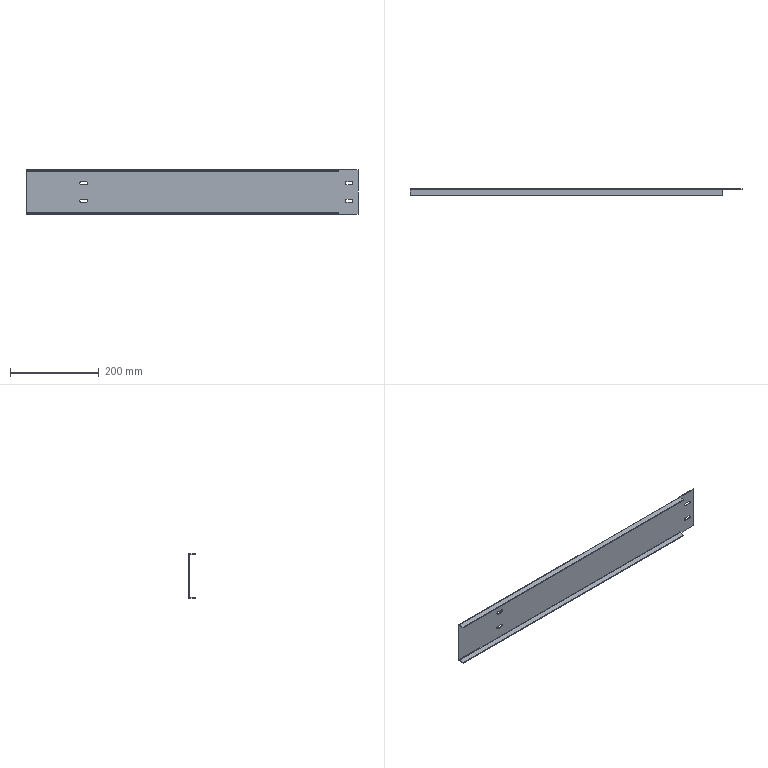Part | STEP file | PN_0006_cover plate | 1 solid | 38 faces | box 750 x 15 x 100 mm | volume 183675 mm3 | plane 26 | cylinder 12 | commonest cylinder face diameters 7 x8 1.473 x2 5.473 x2